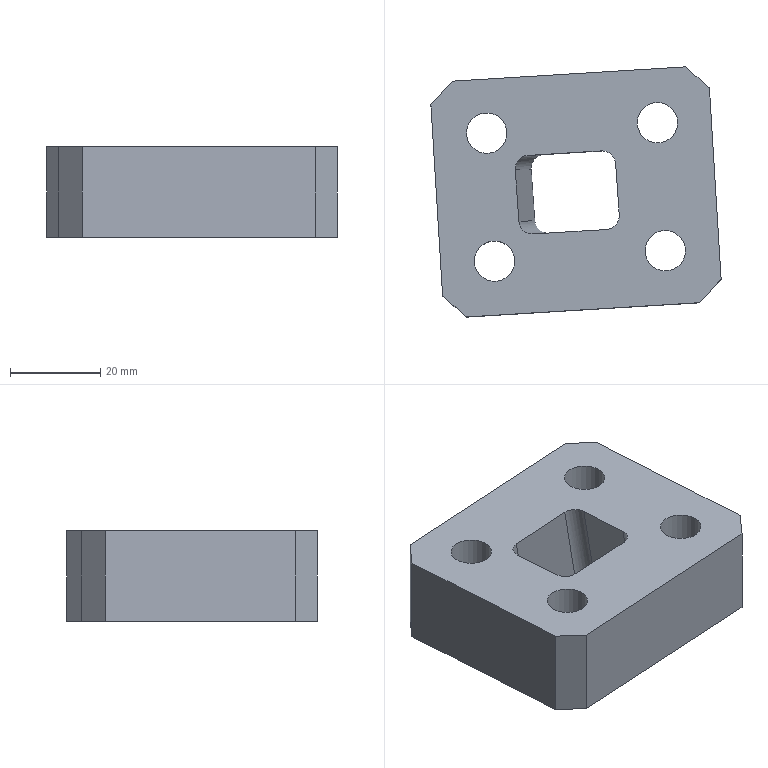Part | STEP file | 车灯-后视镜_id290_x_t | 1 solid | 30 faces | box 64.479 x 55.577 x 20 mm | volume 48278 mm3 | plane 18 | cylinder 12 | commonest cylinder face diameters 6 x4 9 x4 14 x4
STEP:
#1=CARTESIAN_POINT('',(93.683,1.514,-160.5));
#2=VERTEX_POINT('',#1);
#3=CARTESIAN_POINT('',(77.465,0.5225,-160.5));
#4=VERTEX_POINT('',#3);
#5=CARTESIAN_POINT('',(68.963,0.002865,-160.5));
#6=DIRECTION('',(-0.9981,-0.061,0.));
#7=VECTOR('',#6,1.);
#8=LINE('',#5,#7);
#9=EDGE_CURVE('',#2,#4,#8,.T.);
#10=ORIENTED_EDGE('',*,*,#9,.F.);
#11=CARTESIAN_POINT('',(96.539,4.72,-160.5));
#12=VERTEX_POINT('',#11);
#13=CARTESIAN_POINT('',(93.5,4.508,-160.5));
#14=DIRECTION('',(0.,0.,-1.));
#15=DIRECTION('',(-0.9981,-0.061,0.));
#16=AXIS2_PLACEMENT_3D('',#13,#14,#15);
#17=ELLIPSE('',#16,3.046,3.);
#18=EDGE_CURVE('',#12,#2,#17,.T.);
#19=ORIENTED_EDGE('',*,*,#18,.F.);
#20=CARTESIAN_POINT('',(95.736,16.192,-160.5));
#21=VERTEX_POINT('',#20);
#22=CARTESIAN_POINT('',(96.075,11.343,-160.5));
#23=DIRECTION('',(-0.06976,0.9976,0.));
#24=VECTOR('',#23,1.);
#25=LINE('',#22,#24);
#26=EDGE_CURVE('',#12,#21,#25,.T.);
#27=ORIENTED_EDGE('',*,*,#26,.T.);
#28=CARTESIAN_POINT('',(92.514,18.975,-160.5));
#29=VERTEX_POINT('',#28);
#30=CARTESIAN_POINT('',(92.697,15.981,-160.5));
#31=DIRECTION('',(0.,0.,-1.));
#32=DIRECTION('',(0.9981,0.061,0.));
#33=AXIS2_PLACEMENT_3D('',#30,#31,#32);
#34=ELLIPSE('',#33,3.046,3.);
#35=EDGE_CURVE('',#29,#21,#34,.T.);
#36=ORIENTED_EDGE('',*,*,#35,.F.);
#37=CARTESIAN_POINT('',(76.297,17.984,-160.5));
#38=VERTEX_POINT('',#37);
#39=CARTESIAN_POINT('',(67.896,17.47,-160.5));
#40=DIRECTION('',(0.9981,0.061,0.));
#41=VECTOR('',#40,1.);
#42=LINE('',#39,#41);
#43=EDGE_CURVE('',#38,#29,#42,.T.);
#44=ORIENTED_EDGE('',*,*,#43,.F.);
#45=CARTESIAN_POINT('',(73.441,14.778,-160.5));
#46=VERTEX_POINT('',#45);
#47=CARTESIAN_POINT('',(76.48,14.989,-160.5));
#48=DIRECTION('',(0.,0.,-1.));
#49=DIRECTION('',(0.9981,0.061,0.));
#50=AXIS2_PLACEMENT_3D('',#47,#48,#49);
#51=ELLIPSE('',#50,3.046,3.);
#52=EDGE_CURVE('',#46,#38,#51,.T.);
#53=ORIENTED_EDGE('',*,*,#52,.F.);
#54=CARTESIAN_POINT('',(74.244,3.305,-160.5));
#55=VERTEX_POINT('',#54);
#56=CARTESIAN_POINT('',(73.79,9.784,-160.5));
#57=DIRECTION('',(-0.06976,0.9976,0.));
#58=VECTOR('',#57,1.);
#59=LINE('',#56,#58);
#60=EDGE_CURVE('',#55,#46,#59,.T.);
#61=ORIENTED_EDGE('',*,*,#60,.F.);
#62=CARTESIAN_POINT('',(77.282,3.517,-160.5));
#63=DIRECTION('',(0.,0.,-1.));
#64=DIRECTION('',(0.9981,0.061,0.));
#65=AXIS2_PLACEMENT_3D('',#62,#63,#64);
#66=ELLIPSE('',#65,3.046,3.);
#67=EDGE_CURVE('',#4,#55,#66,.T.);
#68=ORIENTED_EDGE('',*,*,#67,.F.);
#69=EDGE_LOOP('',(#10,#19,#27,#36,#44,#53,#61,#68));
#70=FACE_BOUND('',#69,.T.);
#71=CARTESIAN_POINT('',(113.058,32.754,-160.5));
#72=VERTEX_POINT('',#71);
#73=CARTESIAN_POINT('',(115.653,-9.666,-160.5));
#74=VERTEX_POINT('',#73);
#75=CARTESIAN_POINT('',(114.314,12.216,-160.5));
#76=DIRECTION('',(0.06105,-0.9981,0.));
#77=VECTOR('',#76,1.);
#78=LINE('',#75,#77);
#79=EDGE_CURVE('',#72,#74,#78,.T.);
#80=ORIENTED_EDGE('',*,*,#79,.T.);
#81=CARTESIAN_POINT('',(110.967,-14.962,-160.5));
#82=VERTEX_POINT('',#81);
#83=CARTESIAN_POINT('',(115.653,-9.666,-160.5));
#84=DIRECTION('',(0.6626,0.749,0.));
#85=VECTOR('',#84,1.);
#86=LINE('',#83,#85);
#87=EDGE_CURVE('',#82,#74,#86,.T.);
#88=ORIENTED_EDGE('',*,*,#87,.F.);
#89=CARTESIAN_POINT('',(59.064,-18.137,-160.5));
#90=VERTEX_POINT('',#89);
#91=CARTESIAN_POINT('',(70.032,-17.466,-160.5));
#92=DIRECTION('',(-0.9981,-0.06105,0.));
#93=VECTOR('',#92,1.);
#94=LINE('',#91,#93);
#95=EDGE_CURVE('',#82,#90,#94,.T.);
#96=ORIENTED_EDGE('',*,*,#95,.T.);
#97=CARTESIAN_POINT('',(53.768,-13.451,-160.5));
#98=VERTEX_POINT('',#97);
#99=CARTESIAN_POINT('',(53.768,-13.451,-160.5));
#100=DIRECTION('',(0.749,-0.6626,0.));
#101=VECTOR('',#100,1.);
#102=LINE('',#99,#101);
#103=EDGE_CURVE('',#98,#90,#102,.T.);
#104=ORIENTED_EDGE('',*,*,#103,.F.);
#105=CARTESIAN_POINT('',(51.174,28.969,-160.5));
#106=VERTEX_POINT('',#105);
#107=CARTESIAN_POINT('',(52.43,8.431,-160.5));
#108=DIRECTION('',(-0.06105,0.9981,0.));
#109=VECTOR('',#108,1.);
#110=LINE('',#107,#109);
#111=EDGE_CURVE('',#98,#106,#110,.T.);
#112=ORIENTED_EDGE('',*,*,#111,.T.);
#113=CARTESIAN_POINT('',(55.859,34.265,-160.5));
#114=VERTEX_POINT('',#113);
#115=CARTESIAN_POINT('',(51.174,28.969,-160.5));
#116=DIRECTION('',(-0.6626,-0.749,0.));
#117=VECTOR('',#116,1.);
#118=LINE('',#115,#117);
#119=EDGE_CURVE('',#114,#106,#118,.T.);
#120=ORIENTED_EDGE('',*,*,#119,.F.);
#121=CARTESIAN_POINT('',(107.762,37.44,-160.5));
#122=VERTEX_POINT('',#121);
#123=CARTESIAN_POINT('',(66.827,34.936,-160.5));
#124=DIRECTION('',(0.9981,0.06105,0.));
#125=VECTOR('',#124,1.);
#126=LINE('',#123,#125);
#127=EDGE_CURVE('',#114,#122,#126,.T.);
#128=ORIENTED_EDGE('',*,*,#127,.T.);
#129=CARTESIAN_POINT('',(107.762,37.44,-160.5));
#130=DIRECTION('',(-0.749,0.6626,0.));
#131=VECTOR('',#130,1.);
#132=LINE('',#129,#131);
#133=EDGE_CURVE('',#72,#122,#132,.T.);
#134=ORIENTED_EDGE('',*,*,#133,.F.);
#135=EDGE_LOOP('',(#80,#88,#96,#104,#112,#120,#128,#134));
#136=FACE_BOUND('',#135,.T.);
#137=CARTESIAN_POINT('',(58.319,-5.732,-160.5));
#138=VERTEX_POINT('',#137);
#139=CARTESIAN_POINT('',(65.319,-5.732,-160.5));
#140=DIRECTION('',(0.,0.,1.));
#141=DIRECTION('',(-1.,0.,0.));
#142=AXIS2_PLACEMENT_3D('',#139,#140,#141);
#143=CIRCLE('',#142,7.);
#144=EDGE_CURVE('',#138,#138,#143,.T.);
#145=ORIENTED_EDGE('',*,*,#144,.T.);
#146=EDGE_LOOP('',(#145));
#147=FACE_BOUND('',#146,.T.);
#148=CARTESIAN_POINT('',(96.248,-3.412,-160.5));
#149=VERTEX_POINT('',#148);
#150=CARTESIAN_POINT('',(103.248,-3.412,-160.5));
#151=DIRECTION('',(0.,0.,-1.));
#152=DIRECTION('',(-1.,0.,0.));
#153=AXIS2_PLACEMENT_3D('',#150,#151,#152);
#154=CIRCLE('',#153,7.);
#155=EDGE_CURVE('',#149,#149,#154,.T.);
#156=ORIENTED_EDGE('',*,*,#155,.F.);
#157=EDGE_LOOP('',(#156));
#158=FACE_BOUND('',#157,.T.);
#159=CARTESIAN_POINT('',(56.579,22.715,-160.5));
#160=VERTEX_POINT('',#159);
#161=CARTESIAN_POINT('',(63.579,22.715,-160.5));
#162=DIRECTION('',(0.,0.,-1.));
#163=DIRECTION('',(-1.,0.,0.));
#164=AXIS2_PLACEMENT_3D('',#161,#162,#163);
#165=CIRCLE('',#164,7.);
#166=EDGE_CURVE('',#160,#160,#165,.T.);
#167=ORIENTED_EDGE('',*,*,#166,.F.);
#168=EDGE_LOOP('',(#167));
#169=FACE_BOUND('',#168,.T.);
#170=CARTESIAN_POINT('',(94.508,25.035,-160.5));
#171=VERTEX_POINT('',#170);
#172=CARTESIAN_POINT('',(101.508,25.035,-160.5));
#173=DIRECTION('',(0.,0.,1.));
#174=DIRECTION('',(-1.,0.,0.));
#175=AXIS2_PLACEMENT_3D('',#172,#173,#174);
#176=CIRCLE('',#175,7.);
#177=EDGE_CURVE('',#171,#171,#176,.T.);
#178=ORIENTED_EDGE('',*,*,#177,.T.);
#179=EDGE_LOOP('',(#178));
#180=FACE_BOUND('',#179,.T.);
#181=CARTESIAN_POINT('',(68.389,9.407,-160.5));
#182=DIRECTION('',(0.,0.,-1.));
#183=DIRECTION('',(0.9981,0.06105,0.));
#184=AXIS2_PLACEMENT_3D('',#181,#182,#183);
#185=PLANE('',#184);
#186=ADVANCED_FACE('',(#70,#136,#147,#158,#169,#180),#185,.T.);
#187=CARTESIAN_POINT('',(59.064,-18.137,-140.5));
#188=VERTEX_POINT('',#187);
#189=CARTESIAN_POINT('',(110.967,-14.962,-140.5));
#190=VERTEX_POINT('',#189);
#191=CARTESIAN_POINT('',(70.032,-17.466,-140.5));
#192=DIRECTION('',(0.9981,0.06105,0.));
#193=VECTOR('',#192,1.);
#194=LINE('',#191,#193);
#195=EDGE_CURVE('',#188,#190,#194,.T.);
#196=ORIENTED_EDGE('',*,*,#195,.F.);
#197=CARTESIAN_POINT('',(59.064,-18.137,-144.5));
#198=DIRECTION('',(0.,0.,1.));
#199=VECTOR('',#198,1.);
#200=LINE('',#197,#199);
#201=EDGE_CURVE('',#90,#188,#200,.T.);
#202=ORIENTED_EDGE('',*,*,#201,.F.);
#203=ORIENTED_EDGE('',*,*,#95,.F.);
#204=CARTESIAN_POINT('',(110.967,-14.962,-138.5));
#205=DIRECTION('',(0.,0.,-1.));
#206=VECTOR('',#205,1.);
#207=LINE('',#204,#206);
#208=EDGE_CURVE('',#190,#82,#207,.T.);
#209=ORIENTED_EDGE('',*,*,#208,.F.);
#210=EDGE_LOOP('',(#196,#202,#203,#209));
#211=FACE_OUTER_BOUND('',#210,.T.);
#212=CARTESIAN_POINT('',(70.032,-17.466,-138.5));
#213=DIRECTION('',(0.06105,-0.9981,0.));
#214=DIRECTION('',(0.,0.,1.));
#215=AXIS2_PLACEMENT_3D('',#212,#213,#214);
#216=PLANE('',#215);
#217=ADVANCED_FACE('',(#211),#216,.T.);
#218=ORIENTED_EDGE('',*,*,#127,.F.);
#219=CARTESIAN_POINT('',(55.859,34.265,-140.5));
#220=VERTEX_POINT('',#219);
#221=CARTESIAN_POINT('',(55.859,34.265,-144.5));
#222=DIRECTION('',(0.,0.,-1.));
#223=VECTOR('',#222,1.);
#224=LINE('',#221,#223);
#225=EDGE_CURVE('',#220,#114,#224,.T.);
#226=ORIENTED_EDGE('',*,*,#225,.F.);
#227=CARTESIAN_POINT('',(107.762,37.44,-140.5));
#228=VERTEX_POINT('',#227);
#229=CARTESIAN_POINT('',(66.827,34.936,-140.5));
#230=DIRECTION('',(-0.9981,-0.06105,0.));
#231=VECTOR('',#230,1.);
#232=LINE('',#229,#231);
#233=EDGE_CURVE('',#228,#220,#232,.T.);
#234=ORIENTED_EDGE('',*,*,#233,.F.);
#235=CARTESIAN_POINT('',(107.762,37.44,-138.5));
#236=DIRECTION('',(0.,0.,1.));
#237=VECTOR('',#236,1.);
#238=LINE('',#235,#237);
#239=EDGE_CURVE('',#122,#228,#238,.T.);
#240=ORIENTED_EDGE('',*,*,#239,.F.);
#241=EDGE_LOOP('',(#218,#226,#234,#240));
#242=FACE_OUTER_BOUND('',#241,.T.);
#243=CARTESIAN_POINT('',(66.827,34.936,-138.5));
#244=DIRECTION('',(-0.06105,0.9981,0.));
#245=DIRECTION('',(0.,0.,-1.));
#246=AXIS2_PLACEMENT_3D('',#243,#244,#245);
#247=PLANE('',#246);
#248=ADVANCED_FACE('',(#242),#247,.T.);
#249=CARTESIAN_POINT('',(73.945,0.3074,-140.5));
#250=VERTEX_POINT('',#249);
#251=CARTESIAN_POINT('',(90.163,1.299,-140.5));
#252=VERTEX_POINT('',#251);
#253=CARTESIAN_POINT('',(68.963,0.002865,-140.5));
#254=DIRECTION('',(0.9981,0.061,0.));
#255=VECTOR('',#254,1.);
#256=LINE('',#253,#255);
#257=EDGE_CURVE('',#250,#252,#256,.T.);
#258=ORIENTED_EDGE('',*,*,#257,.F.);
#259=CARTESIAN_POINT('',(70.723,3.09,-140.5));
#260=VERTEX_POINT('',#259);
#261=CARTESIAN_POINT('',(73.762,3.302,-140.5));
#262=DIRECTION('',(0.,0.,1.));
#263=DIRECTION('',(0.9981,0.061,0.));
#264=AXIS2_PLACEMENT_3D('',#261,#262,#263);
#265=ELLIPSE('',#264,3.046,3.);
#266=EDGE_CURVE('',#260,#250,#265,.T.);
#267=ORIENTED_EDGE('',*,*,#266,.F.);
#268=CARTESIAN_POINT('',(69.921,14.563,-140.5));
#269=VERTEX_POINT('',#268);
#270=CARTESIAN_POINT('',(70.273,9.538,-140.5));
#271=DIRECTION('',(0.06976,-0.9976,0.));
#272=VECTOR('',#271,1.);
#273=LINE('',#270,#272);
#274=EDGE_CURVE('',#269,#260,#273,.T.);
#275=ORIENTED_EDGE('',*,*,#274,.F.);
#276=CARTESIAN_POINT('',(72.777,17.769,-140.5));
#277=VERTEX_POINT('',#276);
#278=CARTESIAN_POINT('',(72.96,14.774,-140.5));
#279=DIRECTION('',(0.,0.,1.));
#280=DIRECTION('',(0.9981,0.061,0.));
#281=AXIS2_PLACEMENT_3D('',#278,#279,#280);
#282=ELLIPSE('',#281,3.046,3.);
#283=EDGE_CURVE('',#277,#269,#282,.T.);
#284=ORIENTED_EDGE('',*,*,#283,.F.);
#285=CARTESIAN_POINT('',(88.994,18.76,-140.5));
#286=VERTEX_POINT('',#285);
#287=CARTESIAN_POINT('',(67.896,17.47,-140.5));
#288=DIRECTION('',(-0.9981,-0.061,0.));
#289=VECTOR('',#288,1.);
#290=LINE('',#287,#289);
#291=EDGE_CURVE('',#286,#277,#290,.T.);
#292=ORIENTED_EDGE('',*,*,#291,.F.);
#293=CARTESIAN_POINT('',(92.216,15.977,-140.5));
#294=VERTEX_POINT('',#293);
#295=CARTESIAN_POINT('',(89.177,15.765,-140.5));
#296=DIRECTION('',(0.,0.,1.));
#297=DIRECTION('',(0.9981,0.061,0.));
#298=AXIS2_PLACEMENT_3D('',#295,#296,#297);
#299=ELLIPSE('',#298,3.046,3.);
#300=EDGE_CURVE('',#294,#286,#299,.T.);
#301=ORIENTED_EDGE('',*,*,#300,.F.);
#302=CARTESIAN_POINT('',(93.018,4.505,-140.5));
#303=VERTEX_POINT('',#302);
#304=CARTESIAN_POINT('',(92.558,11.097,-140.5));
#305=DIRECTION('',(0.06976,-0.9976,0.));
#306=VECTOR('',#305,1.);
#307=LINE('',#304,#306);
#308=EDGE_CURVE('',#294,#303,#307,.T.);
#309=ORIENTED_EDGE('',*,*,#308,.T.);
#310=CARTESIAN_POINT('',(89.98,4.293,-140.5));
#311=DIRECTION('',(0.,0.,1.));
#312=DIRECTION('',(-0.9981,-0.061,0.));
#313=AXIS2_PLACEMENT_3D('',#310,#311,#312);
#314=ELLIPSE('',#313,3.046,3.);
#315=EDGE_CURVE('',#252,#303,#314,.T.);
#316=ORIENTED_EDGE('',*,*,#315,.F.);
#317=EDGE_LOOP('',(#258,#267,#275,#284,#292,#301,#309,#316));
#318=FACE_BOUND('',#317,.T.);
#319=ORIENTED_EDGE('',*,*,#233,.T.);
#320=CARTESIAN_POINT('',(51.174,28.969,-140.5));
#321=VERTEX_POINT('',#320);
#322=CARTESIAN_POINT('',(51.174,28.969,-140.5));
#323=DIRECTION('',(0.6626,0.749,0.));
#324=VECTOR('',#323,1.);
#325=LINE('',#322,#324);
#326=EDGE_CURVE('',#321,#220,#325,.T.);
#327=ORIENTED_EDGE('',*,*,#326,.F.);
#328=CARTESIAN_POINT('',(53.768,-13.451,-140.5));
#329=VERTEX_POINT('',#328);
#330=CARTESIAN_POINT('',(52.43,8.431,-140.5));
#331=DIRECTION('',(0.06105,-0.9981,0.));
#332=VECTOR('',#331,1.);
#333=LINE('',#330,#332);
#334=EDGE_CURVE('',#321,#329,#333,.T.);
#335=ORIENTED_EDGE('',*,*,#334,.T.);
#336=CARTESIAN_POINT('',(53.768,-13.451,-140.5));
#337=DIRECTION('',(-0.749,0.6626,0.));
#338=VECTOR('',#337,1.);
#339=LINE('',#336,#338);
#340=EDGE_CURVE('',#188,#329,#339,.T.);
#341=ORIENTED_EDGE('',*,*,#340,.F.);
#342=ORIENTED_EDGE('',*,*,#195,.T.);
#343=CARTESIAN_POINT('',(115.653,-9.666,-140.5));
#344=VERTEX_POINT('',#343);
#345=CARTESIAN_POINT('',(115.653,-9.666,-140.5));
#346=DIRECTION('',(-0.6626,-0.749,0.));
#347=VECTOR('',#346,1.);
#348=LINE('',#345,#347);
#349=EDGE_CURVE('',#344,#190,#348,.T.);
#350=ORIENTED_EDGE('',*,*,#349,.F.);
#351=CARTESIAN_POINT('',(113.058,32.754,-140.5));
#352=VERTEX_POINT('',#351);
#353=CARTESIAN_POINT('',(114.314,12.216,-140.5));
#354=DIRECTION('',(-0.06105,0.9981,0.));
#355=VECTOR('',#354,1.);
#356=LINE('',#353,#355);
#357=EDGE_CURVE('',#344,#352,#356,.T.);
#358=ORIENTED_EDGE('',*,*,#357,.T.);
#359=CARTESIAN_POINT('',(107.762,37.44,-140.5));
#360=DIRECTION('',(0.749,-0.6626,0.));
#361=VECTOR('',#360,1.);
#362=LINE('',#359,#361);
#363=EDGE_CURVE('',#228,#352,#362,.T.);
#364=ORIENTED_EDGE('',*,*,#363,.F.);
#365=EDGE_LOOP('',(#319,#327,#335,#341,#342,#350,#358,#364));
#366=FACE_BOUND('',#365,.T.);
#367=CARTESIAN_POINT('',(69.819,-5.732,-140.5));
#368=VERTEX_POINT('',#367);
#369=CARTESIAN_POINT('',(65.319,-5.732,-140.5));
#370=DIRECTION('',(0.,0.,-1.));
#371=DIRECTION('',(1.,0.,0.));
#372=AXIS2_PLACEMENT_3D('',#369,#370,#371);
#373=CIRCLE('',#372,4.5);
#374=EDGE_CURVE('',#368,#368,#373,.T.);
#375=ORIENTED_EDGE('',*,*,#374,.T.);
#376=EDGE_LOOP('',(#375));
#377=FACE_BOUND('',#376,.T.);
#378=CARTESIAN_POINT('',(107.748,-3.412,-140.5));
#379=VERTEX_POINT('',#378);
#380=CARTESIAN_POINT('',(103.248,-3.412,-140.5));
#381=DIRECTION('',(0.,0.,1.));
#382=DIRECTION('',(1.,0.,0.));
#383=AXIS2_PLACEMENT_3D('',#380,#381,#382);
#384=CIRCLE('',#383,4.5);
#385=EDGE_CURVE('',#379,#379,#384,.T.);
#386=ORIENTED_EDGE('',*,*,#385,.F.);
#387=EDGE_LOOP('',(#386));
#388=FACE_BOUND('',#387,.T.);
#389=CARTESIAN_POINT('',(68.079,22.715,-140.5));
#390=VERTEX_POINT('',#389);
#391=CARTESIAN_POINT('',(63.579,22.715,-140.5));
#392=DIRECTION('',(0.,0.,1.));
#393=DIRECTION('',(1.,0.,0.));
#394=AXIS2_PLACEMENT_3D('',#391,#392,#393);
#395=CIRCLE('',#394,4.5);
#396=EDGE_CURVE('',#390,#390,#395,.T.);
#397=ORIENTED_EDGE('',*,*,#396,.F.);
#398=EDGE_LOOP('',(#397));
#399=FACE_BOUND('',#398,.T.);
#400=CARTESIAN_POINT('',(106.008,25.035,-140.5));
#401=VERTEX_POINT('',#400);
#402=CARTESIAN_POINT('',(101.508,25.035,-140.5));
#403=DIRECTION('',(0.,0.,-1.));
#404=DIRECTION('',(1.,0.,0.));
#405=AXIS2_PLACEMENT_3D('',#402,#403,#404);
#406=CIRCLE('',#405,4.5);
#407=EDGE_CURVE('',#401,#401,#406,.T.);
#408=ORIENTED_EDGE('',*,*,#407,.T.);
#409=EDGE_LOOP('',(#408));
#410=FACE_BOUND('',#409,.T.);
#411=CARTESIAN_POINT('',(68.389,9.407,-140.5));
#412=DIRECTION('',(0.,0.,1.));
#413=DIRECTION('',(-0.9981,-0.06105,0.));
#414=AXIS2_PLACEMENT_3D('',#411,#412,#413);
#415=PLANE('',#414);
#416=ADVANCED_FACE('',(#318,#366,#377,#388,#399,#410),#415,.T.);
#417=ORIENTED_EDGE('',*,*,#357,.F.);
#418=CARTESIAN_POINT('',(115.653,-9.666,-138.5));
#419=DIRECTION('',(0.,0.,1.));
#420=VECTOR('',#419,1.);
#421=LINE('',#418,#420);
#422=EDGE_CURVE('',#74,#344,#421,.T.);
#423=ORIENTED_EDGE('',*,*,#422,.F.);
#424=ORIENTED_EDGE('',*,*,#79,.F.);
#425=CARTESIAN_POINT('',(113.058,32.754,-138.5));
#426=DIRECTION('',(0.,0.,-1.));
#427=VECTOR('',#426,1.);
#428=LINE('',#425,#427);
#429=EDGE_CURVE('',#352,#72,#428,.T.);
#430=ORIENTED_EDGE('',*,*,#429,.F.);
#431=EDGE_LOOP('',(#417,#423,#424,#430));
#432=FACE_OUTER_BOUND('',#431,.T.);
#433=CARTESIAN_POINT('',(114.314,12.216,-138.5));
#434=DIRECTION('',(0.9981,0.06105,0.));
#435=DIRECTION('',(0.,0.,1.));
#436=AXIS2_PLACEMENT_3D('',#433,#434,#435);
#437=PLANE('',#436);
#438=ADVANCED_FACE('',(#432),#437,.T.);
#439=CARTESIAN_POINT('',(106.008,25.035,-152.));
#440=VERTEX_POINT('',#439);
#441=CARTESIAN_POINT('',(101.508,25.035,-152.));
#442=DIRECTION('',(0.,0.,-1.));
#443=DIRECTION('',(1.,0.,0.));
#444=AXIS2_PLACEMENT_3D('',#441,#442,#443);
#445=CIRCLE('',#444,4.5);
#446=EDGE_CURVE('',#440,#440,#445,.T.);
#447=ORIENTED_EDGE('',*,*,#446,.T.);
#448=EDGE_LOOP('',(#447));
#449=FACE_BOUND('',#448,.T.);
#450=ORIENTED_EDGE('',*,*,#407,.F.);
#451=EDGE_LOOP('',(#450));
#452=FACE_BOUND('',#451,.T.);
#453=CARTESIAN_POINT('',(101.508,25.035,-140.5));
#454=DIRECTION('',(0.,0.,-1.));
#455=DIRECTION('',(-0.9981,-0.06105,0.));
#456=AXIS2_PLACEMENT_3D('',#453,#454,#455);
#457=CYLINDRICAL_SURFACE('',#456,4.5);
#458=ADVANCED_FACE('',(#449,#452),#457,.F.);
#459=ORIENTED_EDGE('',*,*,#446,.F.);
#460=EDGE_LOOP('',(#459));
#461=FACE_BOUND('',#460,.T.);
#462=CARTESIAN_POINT('',(108.508,25.035,-152.));
#463=VERTEX_POINT('',#462);
#464=CARTESIAN_POINT('',(101.508,25.035,-152.));
#465=DIRECTION('',(0.,0.,-1.));
#466=DIRECTION('',(1.,0.,0.));
#467=AXIS2_PLACEMENT_3D('',#464,#465,#466);
#468=CIRCLE('',#467,7.);
#469=EDGE_CURVE('',#463,#463,#468,.T.);
#470=ORIENTED_EDGE('',*,*,#469,.T.);
#471=EDGE_LOOP('',(#470));
#472=FACE_BOUND('',#471,.T.);
#473=CARTESIAN_POINT('',(101.508,25.035,-152.));
#474=DIRECTION('',(0.,0.,1.));
#475=DIRECTION('',(0.9981,0.06105,0.));
#476=AXIS2_PLACEMENT_3D('',#473,#474,#475);
#477=PLANE('',#476);
#478=ADVANCED_FACE('',(#461,#472),#477,.F.);
#479=ORIENTED_EDGE('',*,*,#469,.F.);
#480=EDGE_LOOP('',(#479));
#481=FACE_BOUND('',#480,.T.);
#482=ORIENTED_EDGE('',*,*,#177,.F.);
#483=EDGE_LOOP('',(#482));
#484=FACE_BOUND('',#483,.T.);
#485=CARTESIAN_POINT('',(101.508,25.035,-150.5));
#486=DIRECTION('',(0.,0.,1.));
#487=DIRECTION('',(0.9981,0.06105,0.));
#488=AXIS2_PLACEMENT_3D('',#485,#486,#487);
#489=CYLINDRICAL_SURFACE('',#488,7.);
#490=ADVANCED_FACE('',(#481,#484),#489,.F.);
#491=CARTESIAN_POINT('',(68.079,22.715,-152.));
#492=VERTEX_POINT('',#491);
#493=CARTESIAN_POINT('',(63.579,22.715,-152.));
#494=DIRECTION('',(0.,0.,1.));
#495=DIRECTION('',(1.,0.,0.));
#496=AXIS2_PLACEMENT_3D('',#493,#494,#495);
#497=CIRCLE('',#496,4.5);
#498=EDGE_CURVE('',#492,#492,#497,.T.);
#499=ORIENTED_EDGE('',*,*,#498,.F.);
#500=EDGE_LOOP('',(#499));
#501=FACE_BOUND('',#500,.T.);
#502=ORIENTED_EDGE('',*,*,#396,.T.);
#503=EDGE_LOOP('',(#502));
#504=FACE_BOUND('',#503,.T.);
#505=CARTESIAN_POINT('',(63.579,22.715,-140.5));
#506=DIRECTION('',(0.,0.,-1.));
#507=DIRECTION('',(0.9981,0.06105,0.));
#508=AXIS2_PLACEMENT_3D('',#505,#506,#507);
#509=CYLINDRICAL_SURFACE('',#508,4.5);
#510=ADVANCED_FACE('',(#501,#504),#509,.F.);
#511=ORIENTED_EDGE('',*,*,#498,.T.);
#512=EDGE_LOOP('',(#511));
#513=FACE_BOUND('',#512,.T.);
#514=CARTESIAN_POINT('',(70.579,22.715,-152.));
#515=VERTEX_POINT('',#514);
#516=CARTESIAN_POINT('',(63.579,22.715,-152.));
#517=DIRECTION('',(0.,0.,1.));
#518=DIRECTION('',(1.,0.,0.));
#519=AXIS2_PLACEMENT_3D('',#516,#517,#518);
#520=CIRCLE('',#519,7.);
#521=EDGE_CURVE('',#515,#515,#520,.T.);
#522=ORIENTED_EDGE('',*,*,#521,.F.);
#523=EDGE_LOOP('',(#522));
#524=FACE_BOUND('',#523,.T.);
#525=CARTESIAN_POINT('',(63.579,22.715,-152.));
#526=DIRECTION('',(0.,0.,1.));
#527=DIRECTION('',(-0.9981,-0.06105,0.));
#528=AXIS2_PLACEMENT_3D('',#525,#526,#527);
#529=PLANE('',#528);
#530=ADVANCED_FACE('',(#513,#524),#529,.F.);
#531=ORIENTED_EDGE('',*,*,#521,.T.);
#532=EDGE_LOOP('',(#531));
#533=FACE_BOUND('',#532,.T.);
#534=ORIENTED_EDGE('',*,*,#166,.T.);
#535=EDGE_LOOP('',(#534));
#536=FACE_BOUND('',#535,.T.);
#537=CARTESIAN_POINT('',(63.579,22.715,-150.5));
#538=DIRECTION('',(0.,0.,1.));
#539=DIRECTION('',(-0.9981,-0.06105,0.));
#540=AXIS2_PLACEMENT_3D('',#537,#538,#539);
#541=CYLINDRICAL_SURFACE('',#540,7.);
#542=ADVANCED_FACE('',(#533,#536),#541,.F.);
#543=CARTESIAN_POINT('',(107.748,-3.412,-152.));
#544=VERTEX_POINT('',#543);
#545=CARTESIAN_POINT('',(103.248,-3.412,-152.));
#546=DIRECTION('',(0.,0.,1.));
#547=DIRECTION('',(1.,0.,0.));
#548=AXIS2_PLACEMENT_3D('',#545,#546,#547);
#549=CIRCLE('',#548,4.5);
#550=EDGE_CURVE('',#544,#544,#549,.T.);
#551=ORIENTED_EDGE('',*,*,#550,.F.);
#552=EDGE_LOOP('',(#551));
#553=FACE_BOUND('',#552,.T.);
#554=ORIENTED_EDGE('',*,*,#385,.T.);
#555=EDGE_LOOP('',(#554));
#556=FACE_BOUND('',#555,.T.);
#557=CARTESIAN_POINT('',(103.248,-3.412,-140.5));
#558=DIRECTION('',(0.,0.,-1.));
#559=DIRECTION('',(-0.9981,-0.06105,0.));
#560=AXIS2_PLACEMENT_3D('',#557,#558,#559);
#561=CYLINDRICAL_SURFACE('',#560,4.5);
#562=ADVANCED_FACE('',(#553,#556),#561,.F.);
#563=ORIENTED_EDGE('',*,*,#550,.T.);
#564=EDGE_LOOP('',(#563));
#565=FACE_BOUND('',#564,.T.);
#566=CARTESIAN_POINT('',(110.248,-3.412,-152.));
#567=VERTEX_POINT('',#566);
#568=CARTESIAN_POINT('',(103.248,-3.412,-152.));
#569=DIRECTION('',(0.,0.,1.));
#570=DIRECTION('',(1.,0.,0.));
#571=AXIS2_PLACEMENT_3D('',#568,#569,#570);
#572=CIRCLE('',#571,7.);
#573=EDGE_CURVE('',#567,#567,#572,.T.);
#574=ORIENTED_EDGE('',*,*,#573,.F.);
#575=EDGE_LOOP('',(#574));
#576=FACE_BOUND('',#575,.T.);
#577=CARTESIAN_POINT('',(103.248,-3.412,-152.));
#578=DIRECTION('',(0.,0.,1.));
#579=DIRECTION('',(0.9981,0.06105,0.));
#580=AXIS2_PLACEMENT_3D('',#577,#578,#579);
#581=PLANE('',#580);
#582=ADVANCED_FACE('',(#565,#576),#581,.F.);
#583=ORIENTED_EDGE('',*,*,#573,.T.);
#584=EDGE_LOOP('',(#583));
#585=FACE_BOUND('',#584,.T.);
#586=ORIENTED_EDGE('',*,*,#155,.T.);
#587=EDGE_LOOP('',(#586));
#588=FACE_BOUND('',#587,.T.);
#589=CARTESIAN_POINT('',(103.248,-3.412,-150.5));
#590=DIRECTION('',(0.,0.,1.));
#591=DIRECTION('',(0.9981,0.06105,0.));
#592=AXIS2_PLACEMENT_3D('',#589,#590,#591);
#593=CYLINDRICAL_SURFACE('',#592,7.);
#594=ADVANCED_FACE('',(#585,#588),#593,.F.);
#595=CARTESIAN_POINT('',(69.819,-5.732,-152.));
#596=VERTEX_POINT('',#595);
#597=CARTESIAN_POINT('',(65.319,-5.732,-152.));
#598=DIRECTION('',(0.,0.,-1.));
#599=DIRECTION('',(1.,0.,0.));
#600=AXIS2_PLACEMENT_3D('',#597,#598,#599);
#601=CIRCLE('',#600,4.5);
#602=EDGE_CURVE('',#596,#596,#601,.T.);
#603=ORIENTED_EDGE('',*,*,#602,.T.);
#604=EDGE_LOOP('',(#603));
#605=FACE_BOUND('',#604,.T.);
#606=ORIENTED_EDGE('',*,*,#374,.F.);
#607=EDGE_LOOP('',(#606));
#608=FACE_BOUND('',#607,.T.);
#609=CARTESIAN_POINT('',(65.319,-5.732,-140.5));
#610=DIRECTION('',(0.,0.,-1.));
#611=DIRECTION('',(0.9981,0.06105,0.));
#612=AXIS2_PLACEMENT_3D('',#609,#610,#611);
#613=CYLINDRICAL_SURFACE('',#612,4.5);
#614=ADVANCED_FACE('',(#605,#608),#613,.F.);
#615=ORIENTED_EDGE('',*,*,#602,.F.);
#616=EDGE_LOOP('',(#615));
#617=FACE_BOUND('',#616,.T.);
#618=CARTESIAN_POINT('',(72.319,-5.732,-152.));
#619=VERTEX_POINT('',#618);
#620=CARTESIAN_POINT('',(65.319,-5.732,-152.));
#621=DIRECTION('',(0.,0.,-1.));
#622=DIRECTION('',(1.,0.,0.));
#623=AXIS2_PLACEMENT_3D('',#620,#621,#622);
#624=CIRCLE('',#623,7.);
#625=EDGE_CURVE('',#619,#619,#624,.T.);
#626=ORIENTED_EDGE('',*,*,#625,.T.);
#627=EDGE_LOOP('',(#626));
#628=FACE_BOUND('',#627,.T.);
#629=CARTESIAN_POINT('',(65.319,-5.732,-152.));
#630=DIRECTION('',(0.,0.,1.));
#631=DIRECTION('',(-0.9981,-0.06105,0.));
#632=AXIS2_PLACEMENT_3D('',#629,#630,#631);
#633=PLANE('',#632);
#634=ADVANCED_FACE('',(#617,#628),#633,.F.);
#635=ORIENTED_EDGE('',*,*,#625,.F.);
#636=EDGE_LOOP('',(#635));
#637=FACE_BOUND('',#636,.T.);
#638=ORIENTED_EDGE('',*,*,#144,.F.);
#639=EDGE_LOOP('',(#638));
#640=FACE_BOUND('',#639,.T.);
#641=CARTESIAN_POINT('',(65.319,-5.732,-150.5));
#642=DIRECTION('',(0.,0.,1.));
#643=DIRECTION('',(-0.9981,-0.06105,0.));
#644=AXIS2_PLACEMENT_3D('',#641,#642,#643);
#645=CYLINDRICAL_SURFACE('',#644,7.);
#646=ADVANCED_FACE('',(#637,#640),#645,.F.);
#647=ORIENTED_EDGE('',*,*,#334,.F.);
#648=CARTESIAN_POINT('',(51.174,28.969,-144.5));
#649=DIRECTION('',(0.,0.,1.));
#650=VECTOR('',#649,1.);
#651=LINE('',#648,#650);
#652=EDGE_CURVE('',#106,#321,#651,.T.);
#653=ORIENTED_EDGE('',*,*,#652,.F.);
#654=ORIENTED_EDGE('',*,*,#111,.F.);
#655=CARTESIAN_POINT('',(53.768,-13.451,-144.5));
#656=DIRECTION('',(0.,0.,-1.));
#657=VECTOR('',#656,1.);
#658=LINE('',#655,#657);
#659=EDGE_CURVE('',#329,#98,#658,.T.);
#660=ORIENTED_EDGE('',*,*,#659,.F.);
#661=EDGE_LOOP('',(#647,#653,#654,#660));
#662=FACE_OUTER_BOUND('',#661,.T.);
#663=CARTESIAN_POINT('',(52.43,8.431,-144.5));
#664=DIRECTION('',(0.9981,0.06105,0.));
#665=DIRECTION('',(0.,0.,-1.));
#666=AXIS2_PLACEMENT_3D('',#663,#664,#665);
#667=PLANE('',#666);
#668=ADVANCED_FACE('',(#662),#667,.F.);
#669=ORIENTED_EDGE('',*,*,#340,.T.);
#670=ORIENTED_EDGE('',*,*,#659,.T.);
#671=ORIENTED_EDGE('',*,*,#103,.T.);
#672=ORIENTED_EDGE('',*,*,#201,.T.);
#673=EDGE_LOOP('',(#669,#670,#671,#672));
#674=FACE_OUTER_BOUND('',#673,.T.);
#675=CARTESIAN_POINT('',(53.768,-13.451,-144.5));
#676=DIRECTION('',(-0.6626,-0.749,0.));
#677=DIRECTION('',(0.749,-0.6626,0.));
#678=AXIS2_PLACEMENT_3D('',#675,#676,#677);
#679=PLANE('',#678);
#680=ADVANCED_FACE('',(#674),#679,.T.);
#681=ORIENTED_EDGE('',*,*,#119,.T.);
#682=ORIENTED_EDGE('',*,*,#652,.T.);
#683=ORIENTED_EDGE('',*,*,#326,.T.);
#684=ORIENTED_EDGE('',*,*,#225,.T.);
#685=EDGE_LOOP('',(#681,#682,#683,#684));
#686=FACE_OUTER_BOUND('',#685,.T.);
#687=CARTESIAN_POINT('',(51.174,28.969,-144.5));
#688=DIRECTION('',(-0.749,0.6626,0.));
#689=DIRECTION('',(-0.6626,-0.749,0.));
#690=AXIS2_PLACEMENT_3D('',#687,#688,#689);
#691=PLANE('',#690);
#692=ADVANCED_FACE('',(#686),#691,.T.);
#693=ORIENTED_EDGE('',*,*,#133,.T.);
#694=ORIENTED_EDGE('',*,*,#239,.T.);
#695=ORIENTED_EDGE('',*,*,#363,.T.);
#696=ORIENTED_EDGE('',*,*,#429,.T.);
#697=EDGE_LOOP('',(#693,#694,#695,#696));
#698=FACE_OUTER_BOUND('',#697,.T.);
#699=CARTESIAN_POINT('',(107.762,37.44,-138.5));
#700=DIRECTION('',(-0.6626,-0.749,0.));
#701=DIRECTION('',(0.749,-0.6626,0.));
#702=AXIS2_PLACEMENT_3D('',#699,#700,#701);
#703=PLANE('',#702);
#704=ADVANCED_FACE('',(#698),#703,.F.);
#705=ORIENTED_EDGE('',*,*,#87,.T.);
#706=ORIENTED_EDGE('',*,*,#422,.T.);
#707=ORIENTED_EDGE('',*,*,#349,.T.);
#708=ORIENTED_EDGE('',*,*,#208,.T.);
#709=EDGE_LOOP('',(#705,#706,#707,#708));
#710=FACE_OUTER_BOUND('',#709,.T.);
#711=CARTESIAN_POINT('',(115.653,-9.666,-138.5));
#712=DIRECTION('',(-0.749,0.6626,0.));
#713=DIRECTION('',(-0.6626,-0.749,0.));
#714=AXIS2_PLACEMENT_3D('',#711,#712,#713);
#715=PLANE('',#714);
#716=ADVANCED_FACE('',(#710),#715,.F.);
#717=ORIENTED_EDGE('',*,*,#9,.T.);
#718=CARTESIAN_POINT('',(49.119,-1.21,0.5535));
#719=DIRECTION('',(0.1733,0.01059,-0.9848));
#720=VECTOR('',#719,1.);
#721=LINE('',#718,#720);
#722=EDGE_CURVE('',#250,#4,#721,.T.);
#723=ORIENTED_EDGE('',*,*,#722,.F.);
#724=ORIENTED_EDGE('',*,*,#257,.T.);
#725=CARTESIAN_POINT('',(59.566,-0.5715,33.339));
#726=DIRECTION('',(-0.1733,-0.01059,0.9848));
#727=VECTOR('',#726,1.);
#728=LINE('',#725,#727);
#729=EDGE_CURVE('',#2,#252,#728,.T.);
#730=ORIENTED_EDGE('',*,*,#729,.F.);
#731=EDGE_LOOP('',(#717,#723,#724,#730));
#732=FACE_OUTER_BOUND('',#731,.T.);
#733=CARTESIAN_POINT('',(67.961,-0.05837,3.882));
#734=DIRECTION('',(0.061,-0.9981,0.));
#735=DIRECTION('',(0.9981,0.061,0.));
#736=AXIS2_PLACEMENT_3D('',#733,#734,#735);
#737=PLANE('',#736);
#738=ADVANCED_FACE('',(#732),#737,.F.);
#739=ORIENTED_EDGE('',*,*,#67,.T.);
#740=CARTESIAN_POINT('',(39.859,1.204,34.859));
#741=DIRECTION('',(-0.1733,-0.01059,0.9848));
#742=VECTOR('',#741,1.);
#743=LINE('',#740,#742);
#744=EDGE_CURVE('',#55,#260,#743,.T.);
#745=ORIENTED_EDGE('',*,*,#744,.T.);
#746=ORIENTED_EDGE('',*,*,#266,.T.);
#747=ORIENTED_EDGE('',*,*,#722,.T.);
#748=EDGE_LOOP('',(#739,#745,#746,#747));
#749=FACE_OUTER_BOUND('',#748,.T.);
#750=CARTESIAN_POINT('',(48.936,1.784,0.5535));
#751=DIRECTION('',(0.1733,0.01059,-0.9848));
#752=DIRECTION('',(-0.9849,0.,-0.1733));
#753=AXIS2_PLACEMENT_3D('',#750,#751,#752);
#754=CYLINDRICAL_SURFACE('',#753,3.);
#755=ADVANCED_FACE('',(#749),#754,.F.);
#756=ORIENTED_EDGE('',*,*,#18,.T.);
#757=ORIENTED_EDGE('',*,*,#729,.T.);
#758=ORIENTED_EDGE('',*,*,#315,.T.);
#759=CARTESIAN_POINT('',(81.688,3.812,-76.122));
#760=DIRECTION('',(0.1733,0.01059,-0.9848));
#761=VECTOR('',#760,1.);
#762=LINE('',#759,#761);
#763=EDGE_CURVE('',#303,#12,#762,.T.);
#764=ORIENTED_EDGE('',*,*,#763,.T.);
#765=EDGE_LOOP('',(#756,#757,#758,#764));
#766=FACE_OUTER_BOUND('',#765,.T.);
#767=CARTESIAN_POINT('',(64.664,2.746,3.332));
#768=DIRECTION('',(-0.1733,-0.01059,0.9848));
#769=DIRECTION('',(0.9849,0.,0.1733));
#770=AXIS2_PLACEMENT_3D('',#767,#768,#769);
#771=CYLINDRICAL_SURFACE('',#770,3.);
#772=ADVANCED_FACE('',(#766),#771,.F.);
#773=ORIENTED_EDGE('',*,*,#60,.T.);
#774=CARTESIAN_POINT('',(39.06,12.676,34.842));
#775=DIRECTION('',(0.1733,0.01059,-0.9848));
#776=VECTOR('',#775,1.);
#777=LINE('',#774,#776);
#778=EDGE_CURVE('',#269,#46,#777,.T.);
#779=ORIENTED_EDGE('',*,*,#778,.F.);
#780=ORIENTED_EDGE('',*,*,#274,.T.);
#781=ORIENTED_EDGE('',*,*,#744,.F.);
#782=EDGE_LOOP('',(#773,#779,#780,#781));
#783=FACE_OUTER_BOUND('',#782,.T.);
#784=CARTESIAN_POINT('',(39.437,7.263,34.85));
#785=DIRECTION('',(-0.9824,-0.0687,-0.1736));
#786=DIRECTION('',(-0.1741,0.,0.9847));
#787=AXIS2_PLACEMENT_3D('',#784,#785,#786);
#788=PLANE('',#787);
#789=ADVANCED_FACE('',(#783),#788,.F.);
#790=ORIENTED_EDGE('',*,*,#52,.T.);
#791=CARTESIAN_POINT('',(47.954,16.251,0.5362));
#792=DIRECTION('',(-0.1733,-0.01059,0.9848));
#793=VECTOR('',#792,1.);
#794=LINE('',#791,#793);
#795=EDGE_CURVE('',#38,#277,#794,.T.);
#796=ORIENTED_EDGE('',*,*,#795,.T.);
#797=ORIENTED_EDGE('',*,*,#283,.T.);
#798=ORIENTED_EDGE('',*,*,#778,.T.);
#799=EDGE_LOOP('',(#790,#796,#797,#798));
#800=FACE_OUTER_BOUND('',#799,.T.);
#801=CARTESIAN_POINT('',(48.137,13.257,0.5362));
#802=DIRECTION('',(0.1733,0.01059,-0.9848));
#803=DIRECTION('',(-0.9849,0.,-0.1733));
#804=AXIS2_PLACEMENT_3D('',#801,#802,#803);
#805=CYLINDRICAL_SURFACE('',#804,3.);
#806=ADVANCED_FACE('',(#800),#805,.F.);
#807=ORIENTED_EDGE('',*,*,#763,.F.);
#808=ORIENTED_EDGE('',*,*,#308,.F.);
#809=CARTESIAN_POINT('',(61.526,14.101,33.869));
#810=DIRECTION('',(-0.1733,-0.01059,0.9848));
#811=VECTOR('',#810,1.);
#812=LINE('',#809,#811);
#813=EDGE_CURVE('',#21,#294,#812,.T.);
#814=ORIENTED_EDGE('',*,*,#813,.F.);
#815=ORIENTED_EDGE('',*,*,#26,.F.);
#816=EDGE_LOOP('',(#807,#808,#814,#815));
#817=FACE_OUTER_BOUND('',#816,.T.);
#818=CARTESIAN_POINT('',(61.892,8.834,33.882));
#819=DIRECTION('',(0.9824,0.0687,0.1736));
#820=DIRECTION('',(0.1741,0.,-0.9847));
#821=AXIS2_PLACEMENT_3D('',#818,#819,#820);
#822=PLANE('',#821);
#823=ADVANCED_FACE('',(#817),#822,.F.);
#824=ORIENTED_EDGE('',*,*,#35,.T.);
#825=ORIENTED_EDGE('',*,*,#813,.T.);
#826=ORIENTED_EDGE('',*,*,#300,.T.);
#827=CARTESIAN_POINT('',(109.326,20.002,-256.016));
#828=DIRECTION('',(0.1733,0.01059,-0.9848));
#829=VECTOR('',#828,1.);
#830=LINE('',#827,#829);
#831=EDGE_CURVE('',#286,#29,#830,.T.);
#832=ORIENTED_EDGE('',*,*,#831,.T.);
#833=EDGE_LOOP('',(#824,#825,#826,#832));
#834=FACE_OUTER_BOUND('',#833,.T.);
#835=CARTESIAN_POINT('',(58.578,13.895,33.353));
#836=DIRECTION('',(0.1733,0.01059,-0.9848));
#837=DIRECTION('',(-0.9849,0.,-0.1733));
#838=AXIS2_PLACEMENT_3D('',#835,#836,#837);
#839=CYLINDRICAL_SURFACE('',#838,3.);
#840=ADVANCED_FACE('',(#834),#839,.F.);
#841=ORIENTED_EDGE('',*,*,#43,.T.);
#842=ORIENTED_EDGE('',*,*,#831,.F.);
#843=ORIENTED_EDGE('',*,*,#291,.T.);
#844=ORIENTED_EDGE('',*,*,#795,.F.);
#845=EDGE_LOOP('',(#841,#842,#843,#844));
#846=FACE_OUTER_BOUND('',#845,.T.);
#847=CARTESIAN_POINT('',(66.894,17.409,3.882));
#848=DIRECTION('',(0.061,-0.9981,0.));
#849=DIRECTION('',(0.9981,0.061,0.));
#850=AXIS2_PLACEMENT_3D('',#847,#848,#849);
#851=PLANE('',#850);
#852=ADVANCED_FACE('',(#846),#851,.T.);
#853=CLOSED_SHELL('',(#186,#217,#248,#416,#438,#458,#478,#490,#510,#530,#542,#562,#582,#594,#614,#634,#646,#668,#680,#692,#704,#716,#738,#755,#772,#789,#806,#823,#840,#852));
#854=MANIFOLD_SOLID_BREP('',#853);
#855=(LENGTH_UNIT()NAMED_UNIT(*)SI_UNIT(.MILLI.,.METRE.));
#856=UNCERTAINTY_MEASURE_WITH_UNIT(LENGTH_MEASURE(0.00002),#855,'','');
#857=(NAMED_UNIT(*)PLANE_ANGLE_UNIT()SI_UNIT($,.RADIAN.));
#858=PLANE_ANGLE_MEASURE_WITH_UNIT(PLANE_ANGLE_MEASURE(0.01745),#857);
#859=DIMENSIONAL_EXPONENTS(0.,0.,0.,0.,0.,0.,0.);
#860=(CONVERSION_BASED_UNIT('DEGREE',#858)NAMED_UNIT(#859)PLANE_ANGLE_UNIT());
#861=(NAMED_UNIT(*)SI_UNIT($,.STERADIAN.)SOLID_ANGLE_UNIT());
#862=(GEOMETRIC_REPRESENTATION_CONTEXT(3)GLOBAL_UNCERTAINTY_ASSIGNED_CONTEXT((#856))GLOBAL_UNIT_ASSIGNED_CONTEXT((#855,#860,#861))REPRESENTATION_CONTEXT('',''));
#863=ADVANCED_BREP_SHAPE_REPRESENTATION('',(#854),#862);